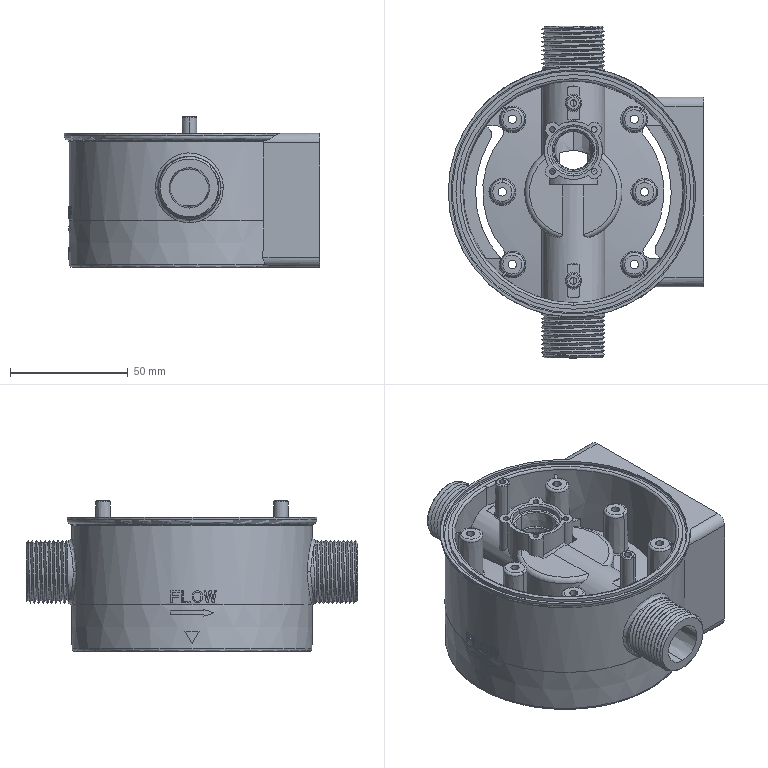Part | NX | features solid 2 | 1 solid | 752 faces | box 108.289 x 140.701 x 63.818 mm | volume 149435 mm3 | cylinder 249 | plane 184 | spline 172 | torus 88 | cone 41 | sphere 18 | commonest cylinder face diameters 2.01 x53 1.005 x46 6.03 x16 3.518 x12 88.038 x12 93.465 x12